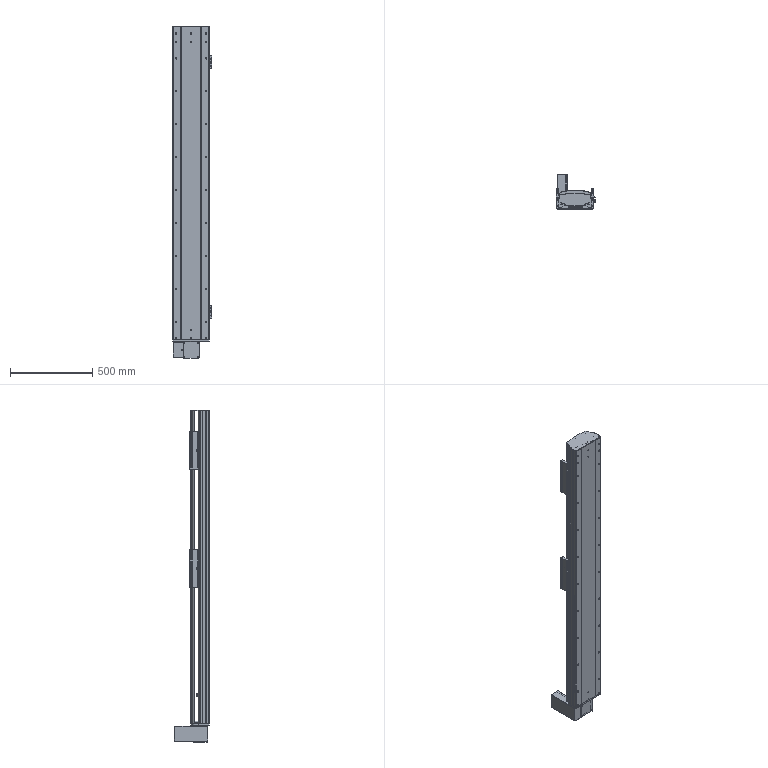Part | SolidWorks | 37 solids | 1824 faces | box 242 x 213.35 x 2015 mm | volume 19740155 mm3 | cylinder 799 | plane 788 | cone 173 | spline 64 | commonest cylinder face diameters 2.5 x64 1 x62 15 x56 6.8 x52 0.5 x48 8.6 x48